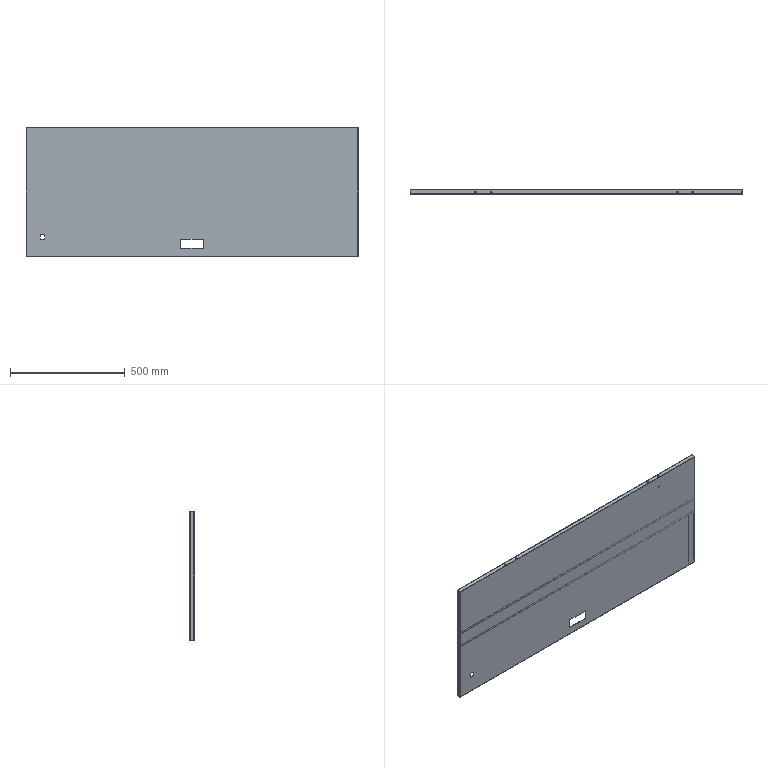Part | SolidWorks | 3 solids | 201 faces | box 1445 x 20 x 561.501 mm | volume 1629553 mm3 | plane 131 | cylinder 62 | spline 8 | commonest cylinder face diameters 0.4 x16 3.3 x16 3.4 x16 8 x8 24 x4 6 x2